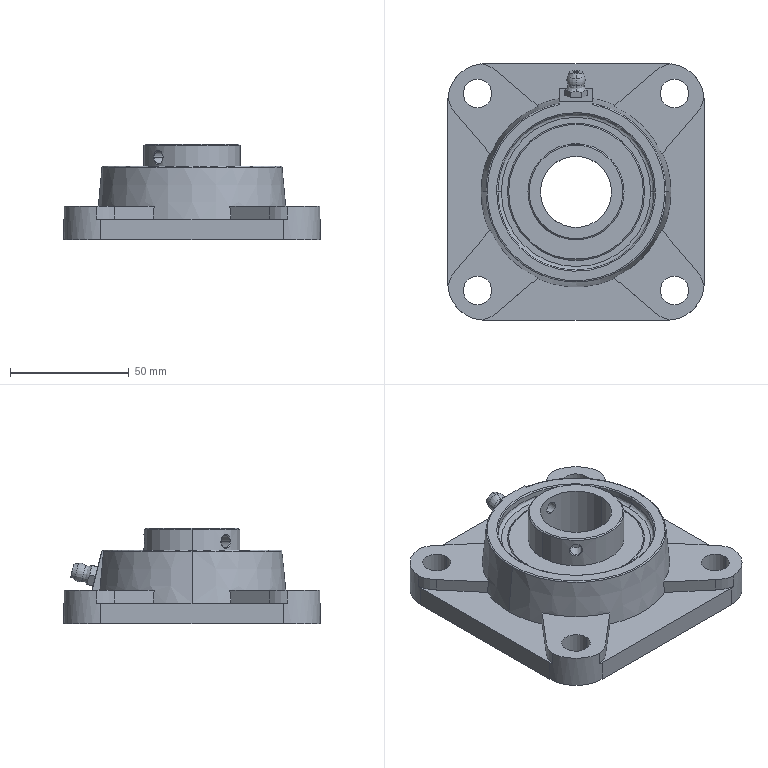Part | SolidWorks | features BaseBody 1 | 1 solid | 107 faces | box 108 x 108 x 40.2 mm | volume 171410 mm3 | cylinder 38 | plane 38 | cone 15 | spline 14 | torus 2 | commonest cylinder face diameters 12 x8 25 x8 5.188 x4 31 x4 40.5 x4 65.882 x4